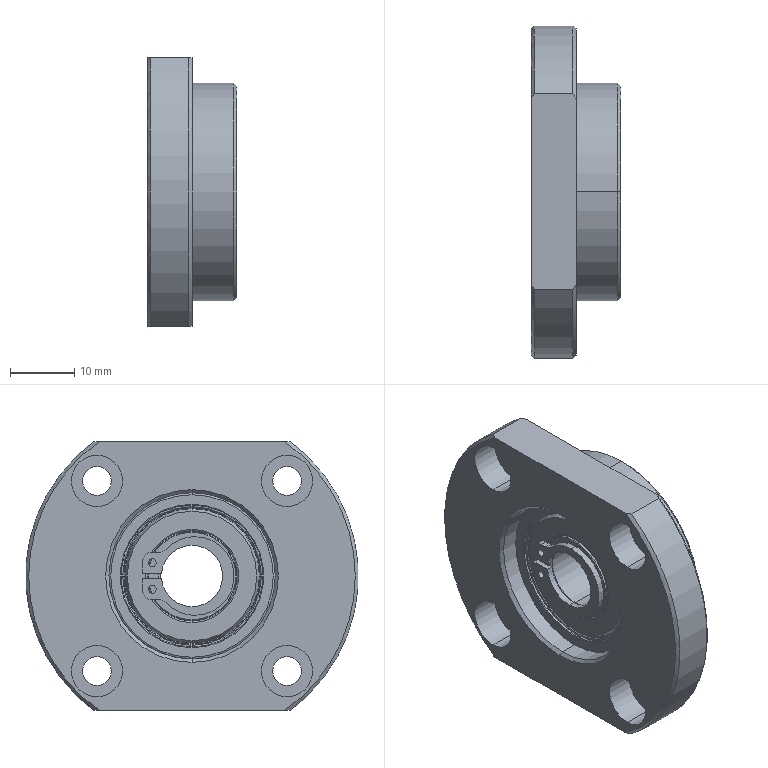Part | STEP file | 001-003-LHF04-R10, | 3 solids | 199 faces | box 14 x 52 x 42 mm | volume 14223 mm3 | cylinder 68 | cone 54 | torus 48 | plane 29 | commonest cylinder face diameters 4.5 x8 8 x8 1.2 x4 3.2 x4 13.3 x4 13.9 x4